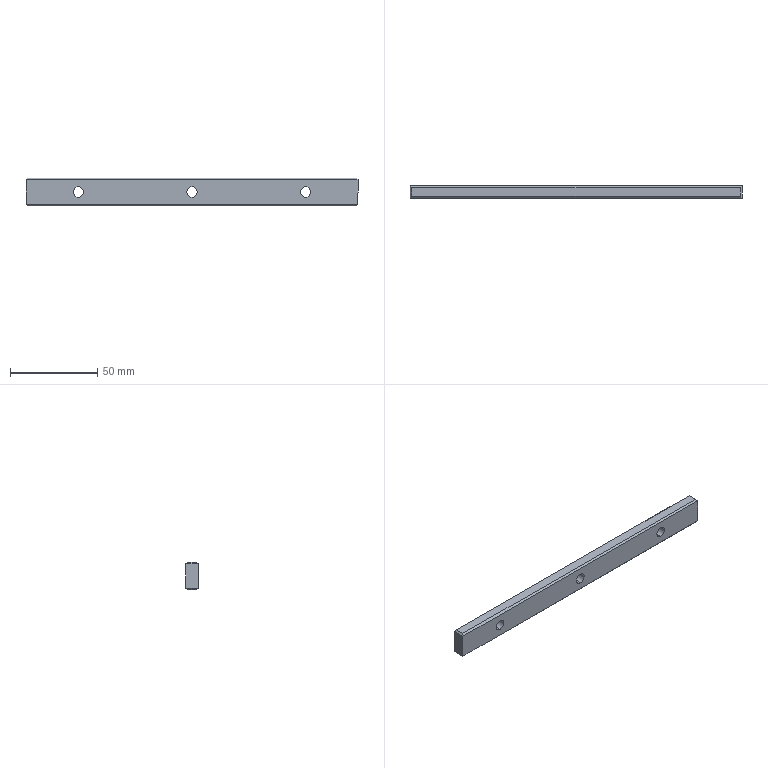Part | SolidWorks | features Chamfer 1, Extrusion 1, HoleWzd 1 | 1 solid | 26 faces | box 190 x 7 x 16 mm | volume 20157 mm3 | plane 14 | cone 6 | cylinder 6 | commonest cylinder face diameters 6 x6
STEP:
#1=CARTESIAN_POINT('',(-65.,1.5,-3.));
#2=VERTEX_POINT('',#1);
#3=CARTESIAN_POINT('',(-65.,1.5,3.));
#4=VERTEX_POINT('',#3);
#5=CARTESIAN_POINT('',(-65.,1.5,0.));
#6=DIRECTION('',(0.,1.,0.));
#7=DIRECTION('',(0.,0.,1.));
#8=AXIS2_PLACEMENT_3D('',#5,#6,#7);
#9=CIRCLE('',#8,3.);
#10=EDGE_CURVE('',#2,#4,#9,.T.);
#11=ORIENTED_EDGE('',*,*,#10,.F.);
#12=CARTESIAN_POINT('',(-65.,3.5,-5.));
#13=VERTEX_POINT('',#12);
#14=CARTESIAN_POINT('',(-65.,3.5,-5.));
#15=DIRECTION('',(0.,0.7071,-0.7071));
#16=VECTOR('',#15,1000.);
#17=LINE('',#14,#16);
#18=EDGE_CURVE('',#2,#13,#17,.T.);
#19=ORIENTED_EDGE('',*,*,#18,.T.);
#20=CARTESIAN_POINT('',(-65.,3.5,5.));
#21=VERTEX_POINT('',#20);
#22=CARTESIAN_POINT('',(-65.,3.5,0.));
#23=DIRECTION('',(0.,1.,0.));
#24=DIRECTION('',(0.,0.,1.));
#25=AXIS2_PLACEMENT_3D('',#22,#23,#24);
#26=CIRCLE('',#25,5.);
#27=EDGE_CURVE('',#13,#21,#26,.T.);
#28=ORIENTED_EDGE('',*,*,#27,.T.);
#29=CARTESIAN_POINT('',(-65.,3.5,5.));
#30=DIRECTION('',(0.,0.7071,0.7071));
#31=VECTOR('',#30,1000.);
#32=LINE('',#29,#31);
#33=EDGE_CURVE('',#4,#21,#32,.T.);
#34=ORIENTED_EDGE('',*,*,#33,.F.);
#35=EDGE_LOOP('',(#11,#19,#28,#34));
#36=FACE_OUTER_BOUND('',#35,.T.);
#37=CARTESIAN_POINT('',(-65.,3.5,0.));
#38=DIRECTION('',(0.,1.,0.));
#39=DIRECTION('',(0.,0.,1.));
#40=AXIS2_PLACEMENT_3D('',#37,#38,#39);
#41=CONICAL_SURFACE('',#40,5.,0.7854);
#42=ADVANCED_FACE('',(#36),#41,.F.);
#43=CARTESIAN_POINT('',(-65.,-3.5,-3.));
#44=VERTEX_POINT('',#43);
#45=CARTESIAN_POINT('',(-65.,-3.5,3.));
#46=VERTEX_POINT('',#45);
#47=CARTESIAN_POINT('',(-65.,-3.5,0.));
#48=DIRECTION('',(0.,1.,0.));
#49=DIRECTION('',(0.,0.,1.));
#50=AXIS2_PLACEMENT_3D('',#47,#48,#49);
#51=CIRCLE('',#50,3.);
#52=EDGE_CURVE('',#44,#46,#51,.T.);
#53=ORIENTED_EDGE('',*,*,#52,.F.);
#54=CARTESIAN_POINT('',(-65.,3.5,-3.));
#55=DIRECTION('',(0.,1.,0.));
#56=VECTOR('',#55,1000.);
#57=LINE('',#54,#56);
#58=EDGE_CURVE('',#44,#2,#57,.T.);
#59=ORIENTED_EDGE('',*,*,#58,.T.);
#60=ORIENTED_EDGE('',*,*,#10,.T.);
#61=CARTESIAN_POINT('',(-65.,3.5,3.));
#62=DIRECTION('',(0.,1.,0.));
#63=VECTOR('',#62,1000.);
#64=LINE('',#61,#63);
#65=EDGE_CURVE('',#46,#4,#64,.T.);
#66=ORIENTED_EDGE('',*,*,#65,.F.);
#67=EDGE_LOOP('',(#53,#59,#60,#66));
#68=FACE_OUTER_BOUND('',#67,.T.);
#69=CARTESIAN_POINT('',(-65.,3.5,0.));
#70=DIRECTION('',(0.,1.,0.));
#71=DIRECTION('',(0.,0.,1.));
#72=AXIS2_PLACEMENT_3D('',#69,#70,#71);
#73=CYLINDRICAL_SURFACE('',#72,3.);
#74=ADVANCED_FACE('',(#68),#73,.F.);
#75=CARTESIAN_POINT('',(0.,1.5,-3.));
#76=VERTEX_POINT('',#75);
#77=CARTESIAN_POINT('',(0.,1.5,3.));
#78=VERTEX_POINT('',#77);
#79=CARTESIAN_POINT('',(0.,1.5,0.));
#80=DIRECTION('',(0.,1.,0.));
#81=DIRECTION('',(0.,0.,1.));
#82=AXIS2_PLACEMENT_3D('',#79,#80,#81);
#83=CIRCLE('',#82,3.);
#84=EDGE_CURVE('',#76,#78,#83,.T.);
#85=ORIENTED_EDGE('',*,*,#84,.F.);
#86=CARTESIAN_POINT('',(0.,3.5,-5.));
#87=VERTEX_POINT('',#86);
#88=CARTESIAN_POINT('',(0.,3.5,-5.));
#89=DIRECTION('',(0.,0.7071,-0.7071));
#90=VECTOR('',#89,1000.);
#91=LINE('',#88,#90);
#92=EDGE_CURVE('',#76,#87,#91,.T.);
#93=ORIENTED_EDGE('',*,*,#92,.T.);
#94=CARTESIAN_POINT('',(0.,3.5,5.));
#95=VERTEX_POINT('',#94);
#96=CARTESIAN_POINT('',(0.,3.5,0.));
#97=DIRECTION('',(0.,1.,0.));
#98=DIRECTION('',(0.,0.,1.));
#99=AXIS2_PLACEMENT_3D('',#96,#97,#98);
#100=CIRCLE('',#99,5.);
#101=EDGE_CURVE('',#87,#95,#100,.T.);
#102=ORIENTED_EDGE('',*,*,#101,.T.);
#103=CARTESIAN_POINT('',(0.,3.5,5.));
#104=DIRECTION('',(0.,0.7071,0.7071));
#105=VECTOR('',#104,1000.);
#106=LINE('',#103,#105);
#107=EDGE_CURVE('',#78,#95,#106,.T.);
#108=ORIENTED_EDGE('',*,*,#107,.F.);
#109=EDGE_LOOP('',(#85,#93,#102,#108));
#110=FACE_OUTER_BOUND('',#109,.T.);
#111=CARTESIAN_POINT('',(0.,3.5,0.));
#112=DIRECTION('',(0.,1.,0.));
#113=DIRECTION('',(0.,0.,1.));
#114=AXIS2_PLACEMENT_3D('',#111,#112,#113);
#115=CONICAL_SURFACE('',#114,5.,0.7854);
#116=ADVANCED_FACE('',(#110),#115,.F.);
#117=CARTESIAN_POINT('',(0.,-3.5,-3.));
#118=VERTEX_POINT('',#117);
#119=CARTESIAN_POINT('',(0.,-3.5,3.));
#120=VERTEX_POINT('',#119);
#121=CARTESIAN_POINT('',(0.,-3.5,0.));
#122=DIRECTION('',(0.,1.,0.));
#123=DIRECTION('',(0.,0.,1.));
#124=AXIS2_PLACEMENT_3D('',#121,#122,#123);
#125=CIRCLE('',#124,3.);
#126=EDGE_CURVE('',#118,#120,#125,.T.);
#127=ORIENTED_EDGE('',*,*,#126,.F.);
#128=CARTESIAN_POINT('',(0.,3.5,-3.));
#129=DIRECTION('',(0.,1.,0.));
#130=VECTOR('',#129,1000.);
#131=LINE('',#128,#130);
#132=EDGE_CURVE('',#118,#76,#131,.T.);
#133=ORIENTED_EDGE('',*,*,#132,.T.);
#134=ORIENTED_EDGE('',*,*,#84,.T.);
#135=CARTESIAN_POINT('',(0.,3.5,3.));
#136=DIRECTION('',(0.,1.,0.));
#137=VECTOR('',#136,1000.);
#138=LINE('',#135,#137);
#139=EDGE_CURVE('',#120,#78,#138,.T.);
#140=ORIENTED_EDGE('',*,*,#139,.F.);
#141=EDGE_LOOP('',(#127,#133,#134,#140));
#142=FACE_OUTER_BOUND('',#141,.T.);
#143=CARTESIAN_POINT('',(0.,3.5,0.));
#144=DIRECTION('',(0.,1.,0.));
#145=DIRECTION('',(0.,0.,1.));
#146=AXIS2_PLACEMENT_3D('',#143,#144,#145);
#147=CYLINDRICAL_SURFACE('',#146,3.);
#148=ADVANCED_FACE('',(#142),#147,.F.);
#149=CARTESIAN_POINT('',(65.,1.5,-3.));
#150=VERTEX_POINT('',#149);
#151=CARTESIAN_POINT('',(65.,1.5,3.));
#152=VERTEX_POINT('',#151);
#153=CARTESIAN_POINT('',(65.,1.5,0.));
#154=DIRECTION('',(0.,1.,0.));
#155=DIRECTION('',(0.,0.,1.));
#156=AXIS2_PLACEMENT_3D('',#153,#154,#155);
#157=CIRCLE('',#156,3.);
#158=EDGE_CURVE('',#150,#152,#157,.T.);
#159=ORIENTED_EDGE('',*,*,#158,.F.);
#160=CARTESIAN_POINT('',(65.,3.5,-5.));
#161=VERTEX_POINT('',#160);
#162=CARTESIAN_POINT('',(65.,3.5,-5.));
#163=DIRECTION('',(0.,0.7071,-0.7071));
#164=VECTOR('',#163,1000.);
#165=LINE('',#162,#164);
#166=EDGE_CURVE('',#150,#161,#165,.T.);
#167=ORIENTED_EDGE('',*,*,#166,.T.);
#168=CARTESIAN_POINT('',(65.,3.5,5.));
#169=VERTEX_POINT('',#168);
#170=CARTESIAN_POINT('',(65.,3.5,0.));
#171=DIRECTION('',(0.,1.,0.));
#172=DIRECTION('',(0.,0.,1.));
#173=AXIS2_PLACEMENT_3D('',#170,#171,#172);
#174=CIRCLE('',#173,5.);
#175=EDGE_CURVE('',#161,#169,#174,.T.);
#176=ORIENTED_EDGE('',*,*,#175,.T.);
#177=CARTESIAN_POINT('',(65.,3.5,5.));
#178=DIRECTION('',(0.,0.7071,0.7071));
#179=VECTOR('',#178,1000.);
#180=LINE('',#177,#179);
#181=EDGE_CURVE('',#152,#169,#180,.T.);
#182=ORIENTED_EDGE('',*,*,#181,.F.);
#183=EDGE_LOOP('',(#159,#167,#176,#182));
#184=FACE_OUTER_BOUND('',#183,.T.);
#185=CARTESIAN_POINT('',(65.,3.5,0.));
#186=DIRECTION('',(0.,1.,0.));
#187=DIRECTION('',(0.,0.,1.));
#188=AXIS2_PLACEMENT_3D('',#185,#186,#187);
#189=CONICAL_SURFACE('',#188,5.,0.7854);
#190=ADVANCED_FACE('',(#184),#189,.F.);
#191=CARTESIAN_POINT('',(65.,-3.5,-3.));
#192=VERTEX_POINT('',#191);
#193=CARTESIAN_POINT('',(65.,-3.5,3.));
#194=VERTEX_POINT('',#193);
#195=CARTESIAN_POINT('',(65.,-3.5,0.));
#196=DIRECTION('',(0.,1.,0.));
#197=DIRECTION('',(0.,0.,1.));
#198=AXIS2_PLACEMENT_3D('',#195,#196,#197);
#199=CIRCLE('',#198,3.);
#200=EDGE_CURVE('',#192,#194,#199,.T.);
#201=ORIENTED_EDGE('',*,*,#200,.F.);
#202=CARTESIAN_POINT('',(65.,3.5,-3.));
#203=DIRECTION('',(0.,1.,0.));
#204=VECTOR('',#203,1000.);
#205=LINE('',#202,#204);
#206=EDGE_CURVE('',#192,#150,#205,.T.);
#207=ORIENTED_EDGE('',*,*,#206,.T.);
#208=ORIENTED_EDGE('',*,*,#158,.T.);
#209=CARTESIAN_POINT('',(65.,3.5,3.));
#210=DIRECTION('',(0.,1.,0.));
#211=VECTOR('',#210,1000.);
#212=LINE('',#209,#211);
#213=EDGE_CURVE('',#194,#152,#212,.T.);
#214=ORIENTED_EDGE('',*,*,#213,.F.);
#215=EDGE_LOOP('',(#201,#207,#208,#214));
#216=FACE_OUTER_BOUND('',#215,.T.);
#217=CARTESIAN_POINT('',(65.,3.5,0.));
#218=DIRECTION('',(0.,1.,0.));
#219=DIRECTION('',(0.,0.,1.));
#220=AXIS2_PLACEMENT_3D('',#217,#218,#219);
#221=CYLINDRICAL_SURFACE('',#220,3.);
#222=ADVANCED_FACE('',(#216),#221,.F.);
#223=CARTESIAN_POINT('',(95.,-3.5,7.));
#224=VERTEX_POINT('',#223);
#225=CARTESIAN_POINT('',(95.,-3.5,-7.));
#226=VERTEX_POINT('',#225);
#227=CARTESIAN_POINT('',(95.,-3.5,-8.));
#228=DIRECTION('',(0.,0.,-1.));
#229=VECTOR('',#228,1000.);
#230=LINE('',#227,#229);
#231=EDGE_CURVE('',#224,#226,#230,.T.);
#232=ORIENTED_EDGE('',*,*,#231,.T.);
#233=CARTESIAN_POINT('',(95.,3.5,-7.));
#234=VERTEX_POINT('',#233);
#235=CARTESIAN_POINT('',(95.,3.5,-7.));
#236=DIRECTION('',(0.,1.,0.));
#237=VECTOR('',#236,1000.);
#238=LINE('',#235,#237);
#239=EDGE_CURVE('',#226,#234,#238,.T.);
#240=ORIENTED_EDGE('',*,*,#239,.T.);
#241=CARTESIAN_POINT('',(95.,3.5,7.));
#242=VERTEX_POINT('',#241);
#243=CARTESIAN_POINT('',(95.,3.5,-8.));
#244=DIRECTION('',(0.,0.,-1.));
#245=VECTOR('',#244,1000.);
#246=LINE('',#243,#245);
#247=EDGE_CURVE('',#242,#234,#246,.T.);
#248=ORIENTED_EDGE('',*,*,#247,.F.);
#249=CARTESIAN_POINT('',(95.,3.5,7.));
#250=DIRECTION('',(0.,-1.,0.));
#251=VECTOR('',#250,1000.);
#252=LINE('',#249,#251);
#253=EDGE_CURVE('',#242,#224,#252,.T.);
#254=ORIENTED_EDGE('',*,*,#253,.T.);
#255=EDGE_LOOP('',(#232,#240,#248,#254));
#256=FACE_OUTER_BOUND('',#255,.T.);
#257=CARTESIAN_POINT('',(95.,3.5,-8.));
#258=DIRECTION('',(-1.,0.,0.));
#259=DIRECTION('',(0.,0.,1.));
#260=AXIS2_PLACEMENT_3D('',#257,#258,#259);
#261=PLANE('',#260);
#262=ADVANCED_FACE('',(#256),#261,.F.);
#263=CARTESIAN_POINT('',(-94.,2.5,-8.));
#264=VERTEX_POINT('',#263);
#265=CARTESIAN_POINT('',(94.,2.5,-8.));
#266=VERTEX_POINT('',#265);
#267=CARTESIAN_POINT('',(95.,2.5,-8.));
#268=DIRECTION('',(1.,0.,0.));
#269=VECTOR('',#268,1000.);
#270=LINE('',#267,#269);
#271=EDGE_CURVE('',#264,#266,#270,.T.);
#272=ORIENTED_EDGE('',*,*,#271,.T.);
#273=CARTESIAN_POINT('',(94.,-2.5,-8.));
#274=VERTEX_POINT('',#273);
#275=CARTESIAN_POINT('',(94.,3.5,-8.));
#276=DIRECTION('',(0.,-1.,0.));
#277=VECTOR('',#276,1000.);
#278=LINE('',#275,#277);
#279=EDGE_CURVE('',#266,#274,#278,.T.);
#280=ORIENTED_EDGE('',*,*,#279,.T.);
#281=CARTESIAN_POINT('',(-94.,-2.5,-8.));
#282=VERTEX_POINT('',#281);
#283=CARTESIAN_POINT('',(-95.,-2.5,-8.));
#284=DIRECTION('',(-1.,0.,0.));
#285=VECTOR('',#284,1000.);
#286=LINE('',#283,#285);
#287=EDGE_CURVE('',#274,#282,#286,.T.);
#288=ORIENTED_EDGE('',*,*,#287,.T.);
#289=CARTESIAN_POINT('',(-94.,3.5,-8.));
#290=DIRECTION('',(0.,1.,0.));
#291=VECTOR('',#290,1000.);
#292=LINE('',#289,#291);
#293=EDGE_CURVE('',#282,#264,#292,.T.);
#294=ORIENTED_EDGE('',*,*,#293,.T.);
#295=EDGE_LOOP('',(#272,#280,#288,#294));
#296=FACE_OUTER_BOUND('',#295,.T.);
#297=CARTESIAN_POINT('',(-95.,3.5,-8.));
#298=DIRECTION('',(0.,0.,1.));
#299=DIRECTION('',(1.,0.,0.));
#300=AXIS2_PLACEMENT_3D('',#297,#298,#299);
#301=PLANE('',#300);
#302=ADVANCED_FACE('',(#296),#301,.F.);
#303=CARTESIAN_POINT('',(-95.,3.5,-7.));
#304=VERTEX_POINT('',#303);
#305=CARTESIAN_POINT('',(-95.,3.5,7.));
#306=VERTEX_POINT('',#305);
#307=CARTESIAN_POINT('',(-95.,3.5,-8.));
#308=DIRECTION('',(0.,0.,1.));
#309=VECTOR('',#308,1000.);
#310=LINE('',#307,#309);
#311=EDGE_CURVE('',#304,#306,#310,.T.);
#312=ORIENTED_EDGE('',*,*,#311,.F.);
#313=CARTESIAN_POINT('',(-95.,-3.5,-7.));
#314=VERTEX_POINT('',#313);
#315=CARTESIAN_POINT('',(-95.,3.5,-7.));
#316=DIRECTION('',(0.,-1.,0.));
#317=VECTOR('',#316,1000.);
#318=LINE('',#315,#317);
#319=EDGE_CURVE('',#304,#314,#318,.T.);
#320=ORIENTED_EDGE('',*,*,#319,.T.);
#321=CARTESIAN_POINT('',(-95.,-3.5,7.));
#322=VERTEX_POINT('',#321);
#323=CARTESIAN_POINT('',(-95.,-3.5,-8.));
#324=DIRECTION('',(0.,0.,1.));
#325=VECTOR('',#324,1000.);
#326=LINE('',#323,#325);
#327=EDGE_CURVE('',#314,#322,#326,.T.);
#328=ORIENTED_EDGE('',*,*,#327,.T.);
#329=CARTESIAN_POINT('',(-95.,3.5,7.));
#330=DIRECTION('',(0.,1.,0.));
#331=VECTOR('',#330,1000.);
#332=LINE('',#329,#331);
#333=EDGE_CURVE('',#322,#306,#332,.T.);
#334=ORIENTED_EDGE('',*,*,#333,.T.);
#335=EDGE_LOOP('',(#312,#320,#328,#334));
#336=FACE_OUTER_BOUND('',#335,.T.);
#337=CARTESIAN_POINT('',(-95.,3.5,-8.));
#338=DIRECTION('',(1.,0.,0.));
#339=DIRECTION('',(0.,0.,-1.));
#340=AXIS2_PLACEMENT_3D('',#337,#338,#339);
#341=PLANE('',#340);
#342=ADVANCED_FACE('',(#336),#341,.F.);
#343=CARTESIAN_POINT('',(94.,2.5,8.));
#344=VERTEX_POINT('',#343);
#345=CARTESIAN_POINT('',(-94.,2.5,8.));
#346=VERTEX_POINT('',#345);
#347=CARTESIAN_POINT('',(-95.,2.5,8.));
#348=DIRECTION('',(-1.,0.,0.));
#349=VECTOR('',#348,1000.);
#350=LINE('',#347,#349);
#351=EDGE_CURVE('',#344,#346,#350,.T.);
#352=ORIENTED_EDGE('',*,*,#351,.T.);
#353=CARTESIAN_POINT('',(-94.,-2.5,8.));
#354=VERTEX_POINT('',#353);
#355=CARTESIAN_POINT('',(-94.,3.5,8.));
#356=DIRECTION('',(0.,-1.,0.));
#357=VECTOR('',#356,1000.);
#358=LINE('',#355,#357);
#359=EDGE_CURVE('',#346,#354,#358,.T.);
#360=ORIENTED_EDGE('',*,*,#359,.T.);
#361=CARTESIAN_POINT('',(94.,-2.5,8.));
#362=VERTEX_POINT('',#361);
#363=CARTESIAN_POINT('',(-95.,-2.5,8.));
#364=DIRECTION('',(1.,0.,0.));
#365=VECTOR('',#364,1000.);
#366=LINE('',#363,#365);
#367=EDGE_CURVE('',#354,#362,#366,.T.);
#368=ORIENTED_EDGE('',*,*,#367,.T.);
#369=CARTESIAN_POINT('',(94.,3.5,8.));
#370=DIRECTION('',(0.,1.,0.));
#371=VECTOR('',#370,1000.);
#372=LINE('',#369,#371);
#373=EDGE_CURVE('',#362,#344,#372,.T.);
#374=ORIENTED_EDGE('',*,*,#373,.T.);
#375=EDGE_LOOP('',(#352,#360,#368,#374));
#376=FACE_OUTER_BOUND('',#375,.T.);
#377=CARTESIAN_POINT('',(-95.,3.5,8.));
#378=DIRECTION('',(0.,0.,-1.));
#379=DIRECTION('',(-1.,0.,0.));
#380=AXIS2_PLACEMENT_3D('',#377,#378,#379);
#381=PLANE('',#380);
#382=ADVANCED_FACE('',(#376),#381,.F.);
#383=CARTESIAN_POINT('',(-65.,3.5,0.));
#384=DIRECTION('',(0.,1.,0.));
#385=DIRECTION('',(0.,0.,1.));
#386=AXIS2_PLACEMENT_3D('',#383,#384,#385);
#387=CIRCLE('',#386,5.);
#388=EDGE_CURVE('',#21,#13,#387,.T.);
#389=ORIENTED_EDGE('',*,*,#388,.F.);
#390=ORIENTED_EDGE('',*,*,#27,.F.);
#391=EDGE_LOOP('',(#389,#390));
#392=FACE_BOUND('',#391,.T.);
#393=CARTESIAN_POINT('',(0.,3.5,0.));
#394=DIRECTION('',(0.,1.,0.));
#395=DIRECTION('',(0.,0.,1.));
#396=AXIS2_PLACEMENT_3D('',#393,#394,#395);
#397=CIRCLE('',#396,5.);
#398=EDGE_CURVE('',#95,#87,#397,.T.);
#399=ORIENTED_EDGE('',*,*,#398,.F.);
#400=ORIENTED_EDGE('',*,*,#101,.F.);
#401=EDGE_LOOP('',(#399,#400));
#402=FACE_BOUND('',#401,.T.);
#403=CARTESIAN_POINT('',(65.,3.5,0.));
#404=DIRECTION('',(0.,1.,0.));
#405=DIRECTION('',(0.,0.,1.));
#406=AXIS2_PLACEMENT_3D('',#403,#404,#405);
#407=CIRCLE('',#406,5.);
#408=EDGE_CURVE('',#169,#161,#407,.T.);
#409=ORIENTED_EDGE('',*,*,#408,.F.);
#410=ORIENTED_EDGE('',*,*,#175,.F.);
#411=EDGE_LOOP('',(#409,#410));
#412=FACE_BOUND('',#411,.T.);
#413=ORIENTED_EDGE('',*,*,#247,.T.);
#414=CARTESIAN_POINT('',(-95.,3.5,-7.));
#415=DIRECTION('',(-1.,0.,0.));
#416=VECTOR('',#415,1000.);
#417=LINE('',#414,#416);
#418=EDGE_CURVE('',#234,#304,#417,.T.);
#419=ORIENTED_EDGE('',*,*,#418,.T.);
#420=ORIENTED_EDGE('',*,*,#311,.T.);
#421=CARTESIAN_POINT('',(95.,3.5,7.));
#422=DIRECTION('',(1.,0.,0.));
#423=VECTOR('',#422,1000.);
#424=LINE('',#421,#423);
#425=EDGE_CURVE('',#306,#242,#424,.T.);
#426=ORIENTED_EDGE('',*,*,#425,.T.);
#427=EDGE_LOOP('',(#413,#419,#420,#426));
#428=FACE_OUTER_BOUND('',#427,.T.);
#429=CARTESIAN_POINT('',(0.,3.5,0.));
#430=DIRECTION('',(0.,1.,0.));
#431=DIRECTION('',(0.,0.,1.));
#432=AXIS2_PLACEMENT_3D('',#429,#430,#431);
#433=PLANE('',#432);
#434=ADVANCED_FACE('',(#392,#402,#412,#428),#433,.T.);
#435=CARTESIAN_POINT('',(-65.,-3.5,0.));
#436=DIRECTION('',(0.,1.,0.));
#437=DIRECTION('',(0.,0.,1.));
#438=AXIS2_PLACEMENT_3D('',#435,#436,#437);
#439=CIRCLE('',#438,3.);
#440=EDGE_CURVE('',#46,#44,#439,.T.);
#441=ORIENTED_EDGE('',*,*,#440,.T.);
#442=ORIENTED_EDGE('',*,*,#52,.T.);
#443=EDGE_LOOP('',(#441,#442));
#444=FACE_BOUND('',#443,.T.);
#445=CARTESIAN_POINT('',(0.,-3.5,0.));
#446=DIRECTION('',(0.,1.,0.));
#447=DIRECTION('',(0.,0.,1.));
#448=AXIS2_PLACEMENT_3D('',#445,#446,#447);
#449=CIRCLE('',#448,3.);
#450=EDGE_CURVE('',#120,#118,#449,.T.);
#451=ORIENTED_EDGE('',*,*,#450,.T.);
#452=ORIENTED_EDGE('',*,*,#126,.T.);
#453=EDGE_LOOP('',(#451,#452));
#454=FACE_BOUND('',#453,.T.);
#455=CARTESIAN_POINT('',(65.,-3.5,0.));
#456=DIRECTION('',(0.,1.,0.));
#457=DIRECTION('',(0.,0.,1.));
#458=AXIS2_PLACEMENT_3D('',#455,#456,#457);
#459=CIRCLE('',#458,3.);
#460=EDGE_CURVE('',#194,#192,#459,.T.);
#461=ORIENTED_EDGE('',*,*,#460,.T.);
#462=ORIENTED_EDGE('',*,*,#200,.T.);
#463=EDGE_LOOP('',(#461,#462));
#464=FACE_BOUND('',#463,.T.);
#465=ORIENTED_EDGE('',*,*,#327,.F.);
#466=CARTESIAN_POINT('',(0.,-3.5,-7.));
#467=DIRECTION('',(1.,0.,0.));
#468=VECTOR('',#467,1000.);
#469=LINE('',#466,#468);
#470=EDGE_CURVE('',#314,#226,#469,.T.);
#471=ORIENTED_EDGE('',*,*,#470,.T.);
#472=ORIENTED_EDGE('',*,*,#231,.F.);
#473=CARTESIAN_POINT('',(0.,-3.5,7.));
#474=DIRECTION('',(-1.,0.,0.));
#475=VECTOR('',#474,1000.);
#476=LINE('',#473,#475);
#477=EDGE_CURVE('',#224,#322,#476,.T.);
#478=ORIENTED_EDGE('',*,*,#477,.T.);
#479=EDGE_LOOP('',(#465,#471,#472,#478));
#480=FACE_OUTER_BOUND('',#479,.T.);
#481=CARTESIAN_POINT('',(0.,-3.5,0.));
#482=DIRECTION('',(0.,1.,0.));
#483=DIRECTION('',(0.,0.,1.));
#484=AXIS2_PLACEMENT_3D('',#481,#482,#483);
#485=PLANE('',#484);
#486=ADVANCED_FACE('',(#444,#454,#464,#480),#485,.F.);
#487=ORIENTED_EDGE('',*,*,#206,.F.);
#488=ORIENTED_EDGE('',*,*,#460,.F.);
#489=ORIENTED_EDGE('',*,*,#213,.T.);
#490=CARTESIAN_POINT('',(65.,1.5,0.));
#491=DIRECTION('',(0.,1.,0.));
#492=DIRECTION('',(0.,0.,1.));
#493=AXIS2_PLACEMENT_3D('',#490,#491,#492);
#494=CIRCLE('',#493,3.);
#495=EDGE_CURVE('',#152,#150,#494,.T.);
#496=ORIENTED_EDGE('',*,*,#495,.T.);
#497=EDGE_LOOP('',(#487,#488,#489,#496));
#498=FACE_OUTER_BOUND('',#497,.T.);
#499=CARTESIAN_POINT('',(65.,3.5,0.));
#500=DIRECTION('',(0.,1.,0.));
#501=DIRECTION('',(0.,0.,1.));
#502=AXIS2_PLACEMENT_3D('',#499,#500,#501);
#503=CYLINDRICAL_SURFACE('',#502,3.);
#504=ADVANCED_FACE('',(#498),#503,.F.);
#505=ORIENTED_EDGE('',*,*,#166,.F.);
#506=ORIENTED_EDGE('',*,*,#495,.F.);
#507=ORIENTED_EDGE('',*,*,#181,.T.);
#508=ORIENTED_EDGE('',*,*,#408,.T.);
#509=EDGE_LOOP('',(#505,#506,#507,#508));
#510=FACE_OUTER_BOUND('',#509,.T.);
#511=CARTESIAN_POINT('',(65.,3.5,0.));
#512=DIRECTION('',(0.,1.,0.));
#513=DIRECTION('',(0.,0.,1.));
#514=AXIS2_PLACEMENT_3D('',#511,#512,#513);
#515=CONICAL_SURFACE('',#514,5.,0.7854);
#516=ADVANCED_FACE('',(#510),#515,.F.);
#517=ORIENTED_EDGE('',*,*,#132,.F.);
#518=ORIENTED_EDGE('',*,*,#450,.F.);
#519=ORIENTED_EDGE('',*,*,#139,.T.);
#520=CARTESIAN_POINT('',(0.,1.5,0.));
#521=DIRECTION('',(0.,1.,0.));
#522=DIRECTION('',(0.,0.,1.));
#523=AXIS2_PLACEMENT_3D('',#520,#521,#522);
#524=CIRCLE('',#523,3.);
#525=EDGE_CURVE('',#78,#76,#524,.T.);
#526=ORIENTED_EDGE('',*,*,#525,.T.);
#527=EDGE_LOOP('',(#517,#518,#519,#526));
#528=FACE_OUTER_BOUND('',#527,.T.);
#529=CARTESIAN_POINT('',(0.,3.5,0.));
#530=DIRECTION('',(0.,1.,0.));
#531=DIRECTION('',(0.,0.,1.));
#532=AXIS2_PLACEMENT_3D('',#529,#530,#531);
#533=CYLINDRICAL_SURFACE('',#532,3.);
#534=ADVANCED_FACE('',(#528),#533,.F.);
#535=ORIENTED_EDGE('',*,*,#92,.F.);
#536=ORIENTED_EDGE('',*,*,#525,.F.);
#537=ORIENTED_EDGE('',*,*,#107,.T.);
#538=ORIENTED_EDGE('',*,*,#398,.T.);
#539=EDGE_LOOP('',(#535,#536,#537,#538));
#540=FACE_OUTER_BOUND('',#539,.T.);
#541=CARTESIAN_POINT('',(0.,3.5,0.));
#542=DIRECTION('',(0.,1.,0.));
#543=DIRECTION('',(0.,0.,1.));
#544=AXIS2_PLACEMENT_3D('',#541,#542,#543);
#545=CONICAL_SURFACE('',#544,5.,0.7854);
#546=ADVANCED_FACE('',(#540),#545,.F.);
#547=ORIENTED_EDGE('',*,*,#58,.F.);
#548=ORIENTED_EDGE('',*,*,#440,.F.);
#549=ORIENTED_EDGE('',*,*,#65,.T.);
#550=CARTESIAN_POINT('',(-65.,1.5,0.));
#551=DIRECTION('',(0.,1.,0.));
#552=DIRECTION('',(0.,0.,1.));
#553=AXIS2_PLACEMENT_3D('',#550,#551,#552);
#554=CIRCLE('',#553,3.);
#555=EDGE_CURVE('',#4,#2,#554,.T.);
#556=ORIENTED_EDGE('',*,*,#555,.T.);
#557=EDGE_LOOP('',(#547,#548,#549,#556));
#558=FACE_OUTER_BOUND('',#557,.T.);
#559=CARTESIAN_POINT('',(-65.,3.5,0.));
#560=DIRECTION('',(0.,1.,0.));
#561=DIRECTION('',(0.,0.,1.));
#562=AXIS2_PLACEMENT_3D('',#559,#560,#561);
#563=CYLINDRICAL_SURFACE('',#562,3.);
#564=ADVANCED_FACE('',(#558),#563,.F.);
#565=ORIENTED_EDGE('',*,*,#18,.F.);
#566=ORIENTED_EDGE('',*,*,#555,.F.);
#567=ORIENTED_EDGE('',*,*,#33,.T.);
#568=ORIENTED_EDGE('',*,*,#388,.T.);
#569=EDGE_LOOP('',(#565,#566,#567,#568));
#570=FACE_OUTER_BOUND('',#569,.T.);
#571=CARTESIAN_POINT('',(-65.,3.5,0.));
#572=DIRECTION('',(0.,1.,0.));
#573=DIRECTION('',(0.,0.,1.));
#574=AXIS2_PLACEMENT_3D('',#571,#572,#573);
#575=CONICAL_SURFACE('',#574,5.,0.7854);
#576=ADVANCED_FACE('',(#570),#575,.F.);
#577=CARTESIAN_POINT('',(-94.333,-2.833,-7.667));
#578=DIRECTION('',(0.5774,0.5774,-0.5774));
#579=VECTOR('',#578,1000.);
#580=LINE('',#577,#579);
#581=EDGE_CURVE('',#314,#282,#580,.T.);
#582=ORIENTED_EDGE('',*,*,#581,.F.);
#583=ORIENTED_EDGE('',*,*,#319,.F.);
#584=CARTESIAN_POINT('',(-95.,3.5,-7.));
#585=DIRECTION('',(-0.5774,0.5774,0.5774));
#586=VECTOR('',#585,1000.);
#587=LINE('',#584,#586);
#588=EDGE_CURVE('',#264,#304,#587,.T.);
#589=ORIENTED_EDGE('',*,*,#588,.F.);
#590=ORIENTED_EDGE('',*,*,#293,.F.);
#591=EDGE_LOOP('',(#582,#583,#589,#590));
#592=FACE_OUTER_BOUND('',#591,.T.);
#593=CARTESIAN_POINT('',(-95.,3.5,-7.));
#594=DIRECTION('',(0.7071,0.,0.7071));
#595=DIRECTION('',(0.,-1.,0.));
#596=AXIS2_PLACEMENT_3D('',#593,#594,#595);
#597=PLANE('',#596);
#598=ADVANCED_FACE('',(#592),#597,.F.);
#599=ORIENTED_EDGE('',*,*,#588,.T.);
#600=ORIENTED_EDGE('',*,*,#418,.F.);
#601=CARTESIAN_POINT('',(63.333,-28.167,-38.667));
#602=DIRECTION('',(0.5774,0.5774,0.5774));
#603=VECTOR('',#602,1000.);
#604=LINE('',#601,#603);
#605=EDGE_CURVE('',#266,#234,#604,.T.);
#606=ORIENTED_EDGE('',*,*,#605,.F.);
#607=ORIENTED_EDGE('',*,*,#271,.F.);
#608=EDGE_LOOP('',(#599,#600,#606,#607));
#609=FACE_OUTER_BOUND('',#608,.T.);
#610=CARTESIAN_POINT('',(0.,3.5,-7.));
#611=DIRECTION('',(0.,0.7071,-0.7071));
#612=DIRECTION('',(1.,0.,0.));
#613=AXIS2_PLACEMENT_3D('',#610,#611,#612);
#614=PLANE('',#613);
#615=ADVANCED_FACE('',(#609),#614,.T.);
#616=ORIENTED_EDGE('',*,*,#581,.T.);
#617=ORIENTED_EDGE('',*,*,#287,.F.);
#618=CARTESIAN_POINT('',(31.,60.5,-71.));
#619=DIRECTION('',(-0.5774,0.5774,-0.5774));
#620=VECTOR('',#619,1000.);
#621=LINE('',#618,#620);
#622=EDGE_CURVE('',#226,#274,#621,.T.);
#623=ORIENTED_EDGE('',*,*,#622,.F.);
#624=ORIENTED_EDGE('',*,*,#470,.F.);
#625=EDGE_LOOP('',(#616,#617,#623,#624));
#626=FACE_OUTER_BOUND('',#625,.T.);
#627=CARTESIAN_POINT('',(-95.,-2.5,-8.));
#628=DIRECTION('',(0.,0.7071,0.7071));
#629=DIRECTION('',(-1.,0.,0.));
#630=AXIS2_PLACEMENT_3D('',#627,#628,#629);
#631=PLANE('',#630);
#632=ADVANCED_FACE('',(#626),#631,.F.);
#633=ORIENTED_EDGE('',*,*,#605,.T.);
#634=ORIENTED_EDGE('',*,*,#239,.F.);
#635=ORIENTED_EDGE('',*,*,#622,.T.);
#636=ORIENTED_EDGE('',*,*,#279,.F.);
#637=EDGE_LOOP('',(#633,#634,#635,#636));
#638=FACE_OUTER_BOUND('',#637,.T.);
#639=CARTESIAN_POINT('',(94.,3.5,-8.));
#640=DIRECTION('',(-0.7071,0.,0.7071));
#641=DIRECTION('',(0.,-1.,0.));
#642=AXIS2_PLACEMENT_3D('',#639,#640,#641);
#643=PLANE('',#642);
#644=ADVANCED_FACE('',(#638),#643,.F.);
#645=CARTESIAN_POINT('',(31.,60.5,71.));
#646=DIRECTION('',(-0.5774,0.5774,0.5774));
#647=VECTOR('',#646,1000.);
#648=LINE('',#645,#647);
#649=EDGE_CURVE('',#224,#362,#648,.T.);
#650=ORIENTED_EDGE('',*,*,#649,.F.);
#651=ORIENTED_EDGE('',*,*,#253,.F.);
#652=CARTESIAN_POINT('',(95.,3.5,7.));
#653=DIRECTION('',(0.5774,0.5774,-0.5774));
#654=VECTOR('',#653,1000.);
#655=LINE('',#652,#654);
#656=EDGE_CURVE('',#344,#242,#655,.T.);
#657=ORIENTED_EDGE('',*,*,#656,.F.);
#658=ORIENTED_EDGE('',*,*,#373,.F.);
#659=EDGE_LOOP('',(#650,#651,#657,#658));
#660=FACE_OUTER_BOUND('',#659,.T.);
#661=CARTESIAN_POINT('',(95.,3.5,7.));
#662=DIRECTION('',(-0.7071,0.,-0.7071));
#663=DIRECTION('',(0.,-1.,0.));
#664=AXIS2_PLACEMENT_3D('',#661,#662,#663);
#665=PLANE('',#664);
#666=ADVANCED_FACE('',(#660),#665,.F.);
#667=ORIENTED_EDGE('',*,*,#656,.T.);
#668=ORIENTED_EDGE('',*,*,#425,.F.);
#669=CARTESIAN_POINT('',(-63.333,-28.167,38.667));
#670=DIRECTION('',(-0.5774,0.5774,-0.5774));
#671=VECTOR('',#670,1000.);
#672=LINE('',#669,#671);
#673=EDGE_CURVE('',#346,#306,#672,.T.);
#674=ORIENTED_EDGE('',*,*,#673,.F.);
#675=ORIENTED_EDGE('',*,*,#351,.F.);
#676=EDGE_LOOP('',(#667,#668,#674,#675));
#677=FACE_OUTER_BOUND('',#676,.T.);
#678=CARTESIAN_POINT('',(0.,3.5,7.));
#679=DIRECTION('',(0.,0.7071,0.7071));
#680=DIRECTION('',(-1.,0.,0.));
#681=AXIS2_PLACEMENT_3D('',#678,#679,#680);
#682=PLANE('',#681);
#683=ADVANCED_FACE('',(#677),#682,.T.);
#684=ORIENTED_EDGE('',*,*,#649,.T.);
#685=ORIENTED_EDGE('',*,*,#367,.F.);
#686=CARTESIAN_POINT('',(-94.333,-2.833,7.667));
#687=DIRECTION('',(0.5774,0.5774,0.5774));
#688=VECTOR('',#687,1000.);
#689=LINE('',#686,#688);
#690=EDGE_CURVE('',#322,#354,#689,.T.);
#691=ORIENTED_EDGE('',*,*,#690,.F.);
#692=ORIENTED_EDGE('',*,*,#477,.F.);
#693=EDGE_LOOP('',(#684,#685,#691,#692));
#694=FACE_OUTER_BOUND('',#693,.T.);
#695=CARTESIAN_POINT('',(-95.,-2.5,8.));
#696=DIRECTION('',(0.,0.7071,-0.7071));
#697=DIRECTION('',(1.,0.,0.));
#698=AXIS2_PLACEMENT_3D('',#695,#696,#697);
#699=PLANE('',#698);
#700=ADVANCED_FACE('',(#694),#699,.F.);
#701=ORIENTED_EDGE('',*,*,#673,.T.);
#702=ORIENTED_EDGE('',*,*,#333,.F.);
#703=ORIENTED_EDGE('',*,*,#690,.T.);
#704=ORIENTED_EDGE('',*,*,#359,.F.);
#705=EDGE_LOOP('',(#701,#702,#703,#704));
#706=FACE_OUTER_BOUND('',#705,.T.);
#707=CARTESIAN_POINT('',(-94.,3.5,8.));
#708=DIRECTION('',(0.7071,0.,-0.7071));
#709=DIRECTION('',(0.,-1.,0.));
#710=AXIS2_PLACEMENT_3D('',#707,#708,#709);
#711=PLANE('',#710);
#712=ADVANCED_FACE('',(#706),#711,.F.);
#713=CLOSED_SHELL('',(#42,#74,#116,#148,#190,#222,#262,#302,#342,#382,#434,#486,#504,#516,#534,#546,#564,#576,#598,#615,#632,#644,#666,#683,#700,#712));
#714=MANIFOLD_SOLID_BREP('',#713);
#715=CARTESIAN_POINT('',(0.,0.,0.));
#716=DIRECTION('',(0.,0.,1.));
#717=DIRECTION('',(1.,0.,0.));
#718=AXIS2_PLACEMENT_3D('',#715,#716,#717);
#719=(LENGTH_UNIT()NAMED_UNIT(*)SI_UNIT(.MILLI.,.METRE.));
#720=UNCERTAINTY_MEASURE_WITH_UNIT(LENGTH_MEASURE(0.00001),#719,'','');
#721=(NAMED_UNIT(*)PLANE_ANGLE_UNIT()SI_UNIT($,.RADIAN.));
#722=(NAMED_UNIT(*)SI_UNIT($,.STERADIAN.)SOLID_ANGLE_UNIT());
#723=(GEOMETRIC_REPRESENTATION_CONTEXT(3)GLOBAL_UNCERTAINTY_ASSIGNED_CONTEXT((#720))GLOBAL_UNIT_ASSIGNED_CONTEXT((#719,#721,#722))REPRESENTATION_CONTEXT('',''));
#724=ADVANCED_BREP_SHAPE_REPRESENTATION('',(#714,#718),#723);